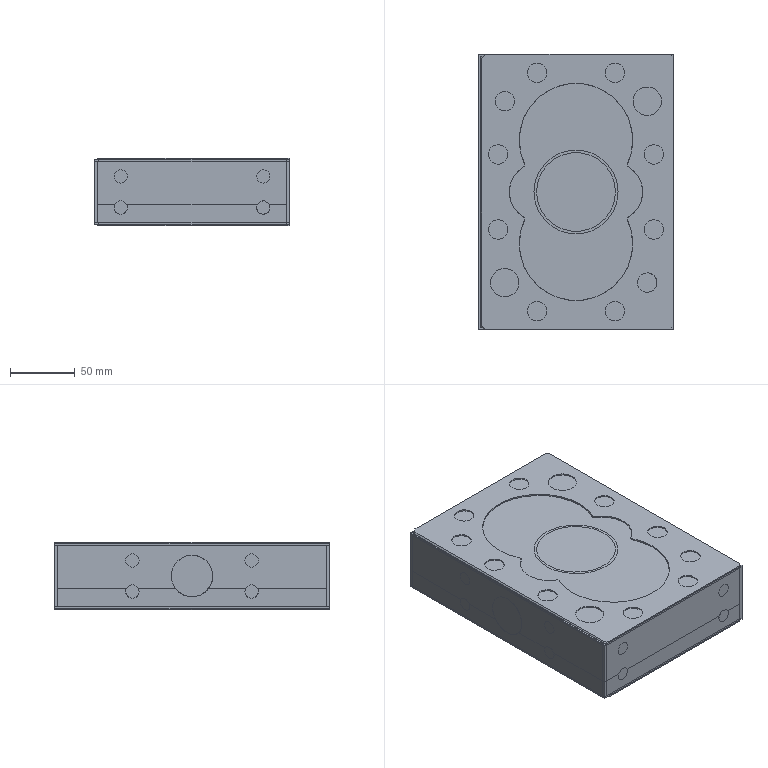NC program | NX | posted with a generic post | part box 150.2 x 212.2 x 52.4 mm
Whole program:
N10 G17 G21 G94 G90
(边界倒角 , TOOL : D6点孔钻)
N12 T06 M6
N14 /M1
N16 G54
N18 G17 G0 G90 X1. Y-77.1 S2000 M3
N20 G43 Z100. H6
N22 Z-1.3
N24 G94 G1 Z-2.3 F400.
N26 G3 X0. Y-76.1 R1.
N28 G1 X-107.1 F500.
N30 Y76.1
N32 X107.1
N34 Y-76.1
N36 X0.
N38 X-0.2
N40 G3 X-1.2 Y-77.1 R1.
N42 G1 Z-1.3
N44 G0 Z100.
(边界倒角_COPY , TOOL : D6点孔钻)
N46 /M1
N48 X-104.607 Y-77.221
N50 Z-1.3
N52 G1 Z-2.3 F400.
N54 G3 X-104.607 Y-75.807 R1.
N56 G1 X-106.807 Y-73.607 F500.
N58 G3 X-108.221 Y-73.607 R1.
N60 G1 Z-1.3
N62 G0 Z100.
N64 Y73.607
N66 Z-1.3
N68 G1 Z-2.3 F400.
N70 G3 X-106.807 Y73.607 R1.
N72 G1 X-104.607 Y75.807 F500.
N74 G3 X-104.607 Y77.221 R1.
N76 G1 Z-1.3
N78 G0 Z100.
N80 X104.607
N82 Z-1.3
N84 G1 Z-2.3 F400.
N86 G3 X104.607 Y75.807 R1.
N88 G1 X106.807 Y73.607 F500.
N90 G3 X108.221 Y73.607 R1.
N92 G1 Z-1.3
N94 G0 Z100.
N96 Y-73.607
N98 Z-1.3
N100 G1 Z-2.3 F400.
N102 G3 X106.807 Y-73.607 R1.
N104 G1 X104.607 Y-75.807 F500.
N106 G3 X104.607 Y-77.221 R1.
N108 G1 Z-1.3
N110 G0 Z100.
N112 M5
N114 M2